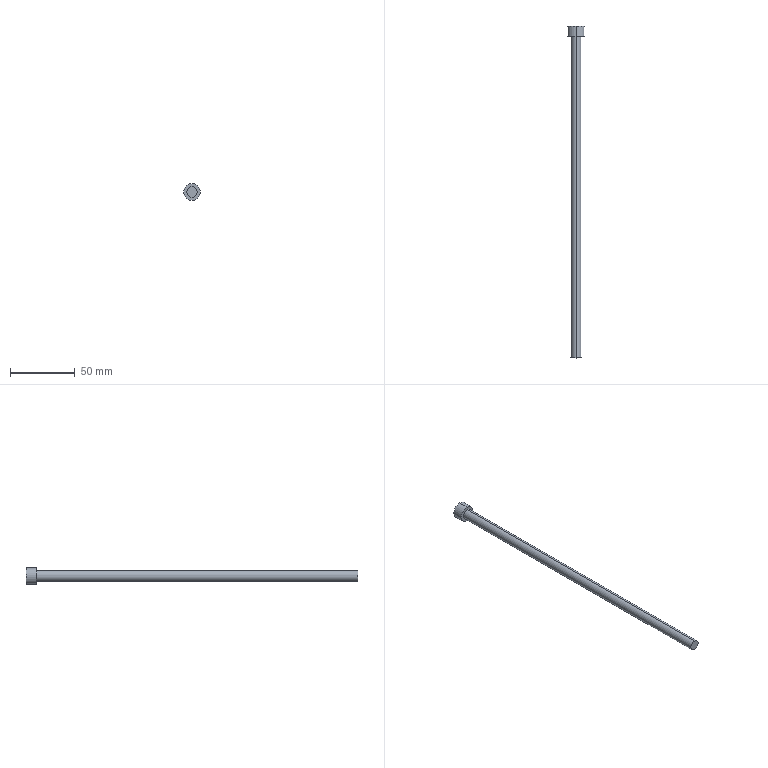Part | STEP file | 1 solid | 7 faces | box 13 x 257.335 x 13 mm | volume 13595 mm3 | cylinder 4 | plane 3 | commonest cylinder face diameters 8 x2 13 x2
STEP:
#1=CARTESIAN_POINT('',(0.,0.,0.));
#2=DIRECTION('',(0.,0.,1.));
#3=DIRECTION('',(1.,0.,0.));
#4=AXIS2_PLACEMENT_3D('',#1,#2,#3);
#5=CARTESIAN_POINT('',(-72.861,290.5,9.027));
#6=VERTEX_POINT('',#5);
#7=CARTESIAN_POINT('',(-72.861,290.5,22.027));
#8=VERTEX_POINT('',#7);
#9=CARTESIAN_POINT('',(-72.861,290.5,15.527));
#10=DIRECTION('',(0.,-1.,0.));
#11=DIRECTION('',(0.,0.,-1.));
#12=AXIS2_PLACEMENT_3D('',#9,#10,#11);
#13=CIRCLE('',#12,6.5);
#14=CARTESIAN_POINT('',(-72.861,290.5,15.527));
#15=DIRECTION('',(0.,-1.,0.));
#16=DIRECTION('',(0.,0.,-1.));
#17=AXIS2_PLACEMENT_3D('',#14,#15,#16);
#18=CYLINDRICAL_SURFACE('',#17,6.5);
#19=CARTESIAN_POINT('',(0.,0.));
#20=DIRECTION('',(1.,0.));
#21=VECTOR('',#20,1.);
#22=LINE('',#19,#21);
#23=(GEOMETRIC_REPRESENTATION_CONTEXT(2)PARAMETRIC_REPRESENTATION_CONTEXT()REPRESENTATION_CONTEXT('',''));
#24=DEFINITIONAL_REPRESENTATION('',(#22),#23);
#25=PCURVE('',#18,#24);
#26=CARTESIAN_POINT('',(-72.862,290.5,110.196));
#27=DIRECTION('',(0.,-1.,0.));
#28=DIRECTION('',(0.,0.,-1.));
#29=AXIS2_PLACEMENT_3D('',#26,#27,#28);
#30=PLANE('',#29);
#31=CARTESIAN_POINT('',(94.669,0.00185));
#32=DIRECTION('',(1.,0.));
#33=AXIS2_PLACEMENT_2D('',#31,#32);
#34=CIRCLE('',#33,6.5);
#35=(GEOMETRIC_REPRESENTATION_CONTEXT(2)PARAMETRIC_REPRESENTATION_CONTEXT()REPRESENTATION_CONTEXT('',''));
#36=DEFINITIONAL_REPRESENTATION('',(#34),#35);
#37=PCURVE('',#30,#36);
#38=SURFACE_CURVE('',#13,(#25,#37),.PCURVE_S1.);
#39=EDGE_CURVE('',#6,#8,#38,.T.);
#40=ORIENTED_EDGE('',*,*,#39,.T.);
#41=CARTESIAN_POINT('',(-72.861,282.5,22.027));
#42=VERTEX_POINT('',#41);
#43=CARTESIAN_POINT('',(-72.861,290.5,22.027));
#44=DIRECTION('',(0.,-1.,0.));
#45=VECTOR('',#44,1.);
#46=LINE('',#43,#45);
#47=CARTESIAN_POINT('',(3.142,0.));
#48=DIRECTION('',(0.,1.));
#49=VECTOR('',#48,1.);
#50=LINE('',#47,#49);
#51=(GEOMETRIC_REPRESENTATION_CONTEXT(2)PARAMETRIC_REPRESENTATION_CONTEXT()REPRESENTATION_CONTEXT('',''));
#52=DEFINITIONAL_REPRESENTATION('',(#50),#51);
#53=PCURVE('',#18,#52);
#54=CARTESIAN_POINT('',(-72.861,290.5,15.527));
#55=DIRECTION('',(0.,-1.,0.));
#56=DIRECTION('',(0.,0.,-1.));
#57=AXIS2_PLACEMENT_3D('',#54,#55,#56);
#58=CYLINDRICAL_SURFACE('',#57,6.5);
#59=CARTESIAN_POINT('',(3.142,0.));
#60=DIRECTION('',(0.,1.));
#61=VECTOR('',#60,1.);
#62=LINE('',#59,#61);
#63=(GEOMETRIC_REPRESENTATION_CONTEXT(2)PARAMETRIC_REPRESENTATION_CONTEXT()REPRESENTATION_CONTEXT('',''));
#64=DEFINITIONAL_REPRESENTATION('',(#62),#63);
#65=PCURVE('',#58,#64);
#66=SURFACE_CURVE('',#46,(#53,#65),.PCURVE_S1.);
#67=EDGE_CURVE('',#8,#42,#66,.T.);
#68=ORIENTED_EDGE('',*,*,#67,.T.);
#69=CARTESIAN_POINT('',(-72.861,282.5,9.027));
#70=VERTEX_POINT('',#69);
#71=CARTESIAN_POINT('',(-72.861,282.5,15.527));
#72=DIRECTION('',(0.,1.,0.));
#73=DIRECTION('',(0.,0.,1.));
#74=AXIS2_PLACEMENT_3D('',#71,#72,#73);
#75=CIRCLE('',#74,6.5);
#76=CARTESIAN_POINT('',(3.142,8.));
#77=DIRECTION('',(-1.,0.));
#78=VECTOR('',#77,1.);
#79=LINE('',#76,#78);
#80=(GEOMETRIC_REPRESENTATION_CONTEXT(2)PARAMETRIC_REPRESENTATION_CONTEXT()REPRESENTATION_CONTEXT('',''));
#81=DEFINITIONAL_REPRESENTATION('',(#79),#80);
#82=PCURVE('',#18,#81);
#83=CARTESIAN_POINT('',(-72.861,282.5,15.527));
#84=DIRECTION('',(0.,-1.,0.));
#85=DIRECTION('',(0.,0.,-1.));
#86=AXIS2_PLACEMENT_3D('',#83,#84,#85);
#87=PLANE('',#86);
#88=CARTESIAN_POINT('',(-6.5,0.));
#89=CARTESIAN_POINT('',(-6.5,11.258));
#90=CARTESIAN_POINT('',(3.25,5.629));
#91=CARTESIAN_POINT('',(13.,0.));
#92=CARTESIAN_POINT('',(3.25,-5.629));
#93=CARTESIAN_POINT('',(-6.5,-11.258));
#94=CARTESIAN_POINT('',(-6.5,0.));
#95=(BOUNDED_CURVE()B_SPLINE_CURVE(2,(#88,#89,#90,#91,#92,#93,#94),.UNSPECIFIED.,.T.,.F.)B_SPLINE_CURVE_WITH_KNOTS((1,2,2,2,2,1),(-2.094,0.,2.094,4.189,6.283,8.378),.UNSPECIFIED.)CURVE()GEOMETRIC_REPRESENTATION_ITEM()RATIONAL_B_SPLINE_CURVE((1.,0.5,1.,0.5,1.,0.5,1.))REPRESENTATION_ITEM(''));
#96=(GEOMETRIC_REPRESENTATION_CONTEXT(2)PARAMETRIC_REPRESENTATION_CONTEXT()REPRESENTATION_CONTEXT('',''));
#97=DEFINITIONAL_REPRESENTATION('',(#95),#96);
#98=PCURVE('',#87,#97);
#99=SURFACE_CURVE('',#75,(#82,#98),.PCURVE_S1.);
#100=EDGE_CURVE('',#42,#70,#99,.T.);
#101=ORIENTED_EDGE('',*,*,#100,.T.);
#102=CARTESIAN_POINT('',(-72.861,290.5,9.027));
#103=DIRECTION('',(0.,-1.,0.));
#104=VECTOR('',#103,1.);
#105=LINE('',#102,#104);
#106=CARTESIAN_POINT('',(0.,0.));
#107=DIRECTION('',(0.,1.));
#108=VECTOR('',#107,1.);
#109=LINE('',#106,#108);
#110=(GEOMETRIC_REPRESENTATION_CONTEXT(2)PARAMETRIC_REPRESENTATION_CONTEXT()REPRESENTATION_CONTEXT('',''));
#111=DEFINITIONAL_REPRESENTATION('',(#109),#110);
#112=PCURVE('',#18,#111);
#113=CARTESIAN_POINT('',(6.283,0.));
#114=DIRECTION('',(0.,1.));
#115=VECTOR('',#114,1.);
#116=LINE('',#113,#115);
#117=(GEOMETRIC_REPRESENTATION_CONTEXT(2)PARAMETRIC_REPRESENTATION_CONTEXT()REPRESENTATION_CONTEXT('',''));
#118=DEFINITIONAL_REPRESENTATION('',(#116),#117);
#119=PCURVE('',#58,#118);
#120=SURFACE_CURVE('',#105,(#112,#119),.PCURVE_S1.);
#121=EDGE_CURVE('',#6,#70,#120,.T.);
#122=ORIENTED_EDGE('',*,*,#121,.F.);
#123=EDGE_LOOP('',(#40,#68,#101,#122));
#124=FACE_BOUND('',#123,.T.);
#125=ADVANCED_FACE('',(#124),#18,.T.);
#126=CARTESIAN_POINT('',(-72.861,282.5,19.527));
#127=VERTEX_POINT('',#126);
#128=CARTESIAN_POINT('',(-72.861,282.5,11.527));
#129=VERTEX_POINT('',#128);
#130=CARTESIAN_POINT('',(-72.861,282.5,15.527));
#131=DIRECTION('',(0.,1.,0.));
#132=DIRECTION('',(0.,0.,-1.));
#133=AXIS2_PLACEMENT_3D('',#130,#131,#132);
#134=CIRCLE('',#133,4.);
#135=CARTESIAN_POINT('',(-72.861,220.5,15.527));
#136=DIRECTION('',(0.,-1.,0.));
#137=DIRECTION('',(0.,0.,-1.));
#138=AXIS2_PLACEMENT_3D('',#135,#136,#137);
#139=CYLINDRICAL_SURFACE('',#138,4.);
#140=CARTESIAN_POINT('',(6.283,-62.));
#141=DIRECTION('',(-1.,0.));
#142=VECTOR('',#141,1.);
#143=LINE('',#140,#142);
#144=(GEOMETRIC_REPRESENTATION_CONTEXT(2)PARAMETRIC_REPRESENTATION_CONTEXT()REPRESENTATION_CONTEXT('',''));
#145=DEFINITIONAL_REPRESENTATION('',(#143),#144);
#146=PCURVE('',#139,#145);
#147=CARTESIAN_POINT('',(4.,0.));
#148=CARTESIAN_POINT('',(4.,-6.928));
#149=CARTESIAN_POINT('',(-2.,-3.464));
#150=CARTESIAN_POINT('',(-8.,0.));
#151=CARTESIAN_POINT('',(-2.,3.464));
#152=CARTESIAN_POINT('',(4.,6.928));
#153=CARTESIAN_POINT('',(4.,0.));
#154=(BOUNDED_CURVE()B_SPLINE_CURVE(2,(#147,#148,#149,#150,#151,#152,#153),.UNSPECIFIED.,.T.,.F.)B_SPLINE_CURVE_WITH_KNOTS((1,2,2,2,2,1),(-2.094,0.,2.094,4.189,6.283,8.378),.UNSPECIFIED.)CURVE()GEOMETRIC_REPRESENTATION_ITEM()RATIONAL_B_SPLINE_CURVE((1.,0.5,1.,0.5,1.,0.5,1.))REPRESENTATION_ITEM(''));
#155=(GEOMETRIC_REPRESENTATION_CONTEXT(2)PARAMETRIC_REPRESENTATION_CONTEXT()REPRESENTATION_CONTEXT('',''));
#156=DEFINITIONAL_REPRESENTATION('',(#154),#155);
#157=PCURVE('',#87,#156);
#158=SURFACE_CURVE('',#134,(#146,#157),.PCURVE_S1.);
#159=EDGE_CURVE('',#127,#129,#158,.T.);
#160=ORIENTED_EDGE('',*,*,#159,.F.);
#161=CARTESIAN_POINT('',(-72.861,33.165,19.527));
#162=VERTEX_POINT('',#161);
#163=CARTESIAN_POINT('',(-72.861,220.5,19.527));
#164=DIRECTION('',(0.,-1.,0.));
#165=VECTOR('',#164,1.);
#166=LINE('',#163,#165);
#167=CARTESIAN_POINT('',(3.142,0.));
#168=DIRECTION('',(0.,1.));
#169=VECTOR('',#168,1.);
#170=LINE('',#167,#169);
#171=(GEOMETRIC_REPRESENTATION_CONTEXT(2)PARAMETRIC_REPRESENTATION_CONTEXT()REPRESENTATION_CONTEXT('',''));
#172=DEFINITIONAL_REPRESENTATION('',(#170),#171);
#173=PCURVE('',#139,#172);
#174=CARTESIAN_POINT('',(-72.861,220.5,15.527));
#175=DIRECTION('',(0.,-1.,0.));
#176=DIRECTION('',(0.,0.,-1.));
#177=AXIS2_PLACEMENT_3D('',#174,#175,#176);
#178=CYLINDRICAL_SURFACE('',#177,4.);
#179=CARTESIAN_POINT('',(3.142,0.));
#180=DIRECTION('',(0.,1.));
#181=VECTOR('',#180,1.);
#182=LINE('',#179,#181);
#183=(GEOMETRIC_REPRESENTATION_CONTEXT(2)PARAMETRIC_REPRESENTATION_CONTEXT()REPRESENTATION_CONTEXT('',''));
#184=DEFINITIONAL_REPRESENTATION('',(#182),#183);
#185=PCURVE('',#178,#184);
#186=SURFACE_CURVE('',#166,(#173,#185),.PCURVE_S1.);
#187=EDGE_CURVE('',#127,#162,#186,.T.);
#188=ORIENTED_EDGE('',*,*,#187,.T.);
#189=CARTESIAN_POINT('',(-72.861,33.165,11.527));
#190=VERTEX_POINT('',#189);
#191=CARTESIAN_POINT('',(-72.861,33.165,15.527));
#192=DIRECTION('',(0.,1.,0.));
#193=DIRECTION('',(0.,0.,-1.));
#194=AXIS2_PLACEMENT_3D('',#191,#192,#193);
#195=CIRCLE('',#194,4.);
#196=CARTESIAN_POINT('',(6.283,187.335));
#197=DIRECTION('',(-1.,0.));
#198=VECTOR('',#197,1.);
#199=LINE('',#196,#198);
#200=(GEOMETRIC_REPRESENTATION_CONTEXT(2)PARAMETRIC_REPRESENTATION_CONTEXT()REPRESENTATION_CONTEXT('',''));
#201=DEFINITIONAL_REPRESENTATION('',(#199),#200);
#202=PCURVE('',#139,#201);
#203=CARTESIAN_POINT('',(-4.271,33.165,10.143));
#204=DIRECTION('',(0.,-1.,0.));
#205=DIRECTION('',(0.,0.,-1.));
#206=AXIS2_PLACEMENT_3D('',#203,#204,#205);
#207=PLANE('',#206);
#208=CARTESIAN_POINT('',(-1.384,-68.589));
#209=CARTESIAN_POINT('',(-1.384,-75.518));
#210=CARTESIAN_POINT('',(-7.384,-72.054));
#211=CARTESIAN_POINT('',(-13.384,-68.589));
#212=CARTESIAN_POINT('',(-7.384,-65.125));
#213=CARTESIAN_POINT('',(-1.384,-61.661));
#214=CARTESIAN_POINT('',(-1.384,-68.589));
#215=(BOUNDED_CURVE()B_SPLINE_CURVE(2,(#208,#209,#210,#211,#212,#213,#214),.UNSPECIFIED.,.T.,.F.)B_SPLINE_CURVE_WITH_KNOTS((1,2,2,2,2,1),(-2.094,0.,2.094,4.189,6.283,8.378),.UNSPECIFIED.)CURVE()GEOMETRIC_REPRESENTATION_ITEM()RATIONAL_B_SPLINE_CURVE((1.,0.5,1.,0.5,1.,0.5,1.))REPRESENTATION_ITEM(''));
#216=(GEOMETRIC_REPRESENTATION_CONTEXT(2)PARAMETRIC_REPRESENTATION_CONTEXT()REPRESENTATION_CONTEXT('',''));
#217=DEFINITIONAL_REPRESENTATION('',(#215),#216);
#218=PCURVE('',#207,#217);
#219=SURFACE_CURVE('',#195,(#202,#218),.PCURVE_S1.);
#220=EDGE_CURVE('',#162,#190,#219,.T.);
#221=ORIENTED_EDGE('',*,*,#220,.T.);
#222=CARTESIAN_POINT('',(-72.861,220.5,11.527));
#223=DIRECTION('',(0.,-1.,0.));
#224=VECTOR('',#223,1.);
#225=LINE('',#222,#224);
#226=CARTESIAN_POINT('',(0.,0.));
#227=DIRECTION('',(0.,1.));
#228=VECTOR('',#227,1.);
#229=LINE('',#226,#228);
#230=(GEOMETRIC_REPRESENTATION_CONTEXT(2)PARAMETRIC_REPRESENTATION_CONTEXT()REPRESENTATION_CONTEXT('',''));
#231=DEFINITIONAL_REPRESENTATION('',(#229),#230);
#232=PCURVE('',#139,#231);
#233=CARTESIAN_POINT('',(6.283,0.));
#234=DIRECTION('',(0.,1.));
#235=VECTOR('',#234,1.);
#236=LINE('',#233,#235);
#237=(GEOMETRIC_REPRESENTATION_CONTEXT(2)PARAMETRIC_REPRESENTATION_CONTEXT()REPRESENTATION_CONTEXT('',''));
#238=DEFINITIONAL_REPRESENTATION('',(#236),#237);
#239=PCURVE('',#178,#238);
#240=SURFACE_CURVE('',#225,(#232,#239),.PCURVE_S1.);
#241=EDGE_CURVE('',#129,#190,#240,.T.);
#242=ORIENTED_EDGE('',*,*,#241,.F.);
#243=EDGE_LOOP('',(#160,#188,#221,#242));
#244=FACE_BOUND('',#243,.T.);
#245=ADVANCED_FACE('',(#244),#139,.T.);
#246=ORIENTED_EDGE('',*,*,#187,.F.);
#247=CARTESIAN_POINT('',(-72.861,282.5,15.527));
#248=DIRECTION('',(0.,1.,0.));
#249=DIRECTION('',(0.,0.,-1.));
#250=AXIS2_PLACEMENT_3D('',#247,#248,#249);
#251=CIRCLE('',#250,4.);
#252=CARTESIAN_POINT('',(6.283,-62.));
#253=DIRECTION('',(-1.,0.));
#254=VECTOR('',#253,1.);
#255=LINE('',#252,#254);
#256=(GEOMETRIC_REPRESENTATION_CONTEXT(2)PARAMETRIC_REPRESENTATION_CONTEXT()REPRESENTATION_CONTEXT('',''));
#257=DEFINITIONAL_REPRESENTATION('',(#255),#256);
#258=PCURVE('',#178,#257);
#259=CARTESIAN_POINT('',(4.,0.));
#260=CARTESIAN_POINT('',(4.,-6.928));
#261=CARTESIAN_POINT('',(-2.,-3.464));
#262=CARTESIAN_POINT('',(-8.,0.));
#263=CARTESIAN_POINT('',(-2.,3.464));
#264=CARTESIAN_POINT('',(4.,6.928));
#265=CARTESIAN_POINT('',(4.,0.));
#266=(BOUNDED_CURVE()B_SPLINE_CURVE(2,(#259,#260,#261,#262,#263,#264,#265),.UNSPECIFIED.,.T.,.F.)B_SPLINE_CURVE_WITH_KNOTS((1,2,2,2,2,1),(-2.094,0.,2.094,4.189,6.283,8.378),.UNSPECIFIED.)CURVE()GEOMETRIC_REPRESENTATION_ITEM()RATIONAL_B_SPLINE_CURVE((1.,0.5,1.,0.5,1.,0.5,1.))REPRESENTATION_ITEM(''));
#267=(GEOMETRIC_REPRESENTATION_CONTEXT(2)PARAMETRIC_REPRESENTATION_CONTEXT()REPRESENTATION_CONTEXT('',''));
#268=DEFINITIONAL_REPRESENTATION('',(#266),#267);
#269=PCURVE('',#87,#268);
#270=SURFACE_CURVE('',#251,(#258,#269),.PCURVE_S1.);
#271=EDGE_CURVE('',#129,#127,#270,.T.);
#272=ORIENTED_EDGE('',*,*,#271,.F.);
#273=ORIENTED_EDGE('',*,*,#241,.T.);
#274=CARTESIAN_POINT('',(-72.861,33.165,15.527));
#275=DIRECTION('',(0.,1.,0.));
#276=DIRECTION('',(0.,0.,-1.));
#277=AXIS2_PLACEMENT_3D('',#274,#275,#276);
#278=CIRCLE('',#277,4.);
#279=CARTESIAN_POINT('',(6.283,187.335));
#280=DIRECTION('',(-1.,0.));
#281=VECTOR('',#280,1.);
#282=LINE('',#279,#281);
#283=(GEOMETRIC_REPRESENTATION_CONTEXT(2)PARAMETRIC_REPRESENTATION_CONTEXT()REPRESENTATION_CONTEXT('',''));
#284=DEFINITIONAL_REPRESENTATION('',(#282),#283);
#285=PCURVE('',#178,#284);
#286=CARTESIAN_POINT('',(-1.384,-68.589));
#287=CARTESIAN_POINT('',(-1.384,-75.518));
#288=CARTESIAN_POINT('',(-7.384,-72.054));
#289=CARTESIAN_POINT('',(-13.384,-68.589));
#290=CARTESIAN_POINT('',(-7.384,-65.125));
#291=CARTESIAN_POINT('',(-1.384,-61.661));
#292=CARTESIAN_POINT('',(-1.384,-68.589));
#293=(BOUNDED_CURVE()B_SPLINE_CURVE(2,(#286,#287,#288,#289,#290,#291,#292),.UNSPECIFIED.,.T.,.F.)B_SPLINE_CURVE_WITH_KNOTS((1,2,2,2,2,1),(-2.094,0.,2.094,4.189,6.283,8.378),.UNSPECIFIED.)CURVE()GEOMETRIC_REPRESENTATION_ITEM()RATIONAL_B_SPLINE_CURVE((1.,0.5,1.,0.5,1.,0.5,1.))REPRESENTATION_ITEM(''));
#294=(GEOMETRIC_REPRESENTATION_CONTEXT(2)PARAMETRIC_REPRESENTATION_CONTEXT()REPRESENTATION_CONTEXT('',''));
#295=DEFINITIONAL_REPRESENTATION('',(#293),#294);
#296=PCURVE('',#207,#295);
#297=SURFACE_CURVE('',#278,(#285,#296),.PCURVE_S1.);
#298=EDGE_CURVE('',#190,#162,#297,.T.);
#299=ORIENTED_EDGE('',*,*,#298,.T.);
#300=EDGE_LOOP('',(#246,#272,#273,#299));
#301=FACE_BOUND('',#300,.T.);
#302=ADVANCED_FACE('',(#301),#178,.T.);
#303=ORIENTED_EDGE('',*,*,#298,.F.);
#304=ORIENTED_EDGE('',*,*,#220,.F.);
#305=EDGE_LOOP('',(#303,#304));
#306=FACE_BOUND('',#305,.T.);
#307=ADVANCED_FACE('',(#306),#207,.T.);
#308=ORIENTED_EDGE('',*,*,#271,.T.);
#309=ORIENTED_EDGE('',*,*,#159,.T.);
#310=EDGE_LOOP('',(#308,#309));
#311=FACE_BOUND('',#310,.T.);
#312=CARTESIAN_POINT('',(-72.861,282.5,15.527));
#313=DIRECTION('',(0.,1.,0.));
#314=DIRECTION('',(0.,0.,1.));
#315=AXIS2_PLACEMENT_3D('',#312,#313,#314);
#316=CIRCLE('',#315,6.5);
#317=CARTESIAN_POINT('',(-6.5,0.));
#318=CARTESIAN_POINT('',(-6.5,11.258));
#319=CARTESIAN_POINT('',(3.25,5.629));
#320=CARTESIAN_POINT('',(13.,0.));
#321=CARTESIAN_POINT('',(3.25,-5.629));
#322=CARTESIAN_POINT('',(-6.5,-11.258));
#323=CARTESIAN_POINT('',(-6.5,0.));
#324=(BOUNDED_CURVE()B_SPLINE_CURVE(2,(#317,#318,#319,#320,#321,#322,#323),.UNSPECIFIED.,.T.,.F.)B_SPLINE_CURVE_WITH_KNOTS((1,2,2,2,2,1),(-2.094,0.,2.094,4.189,6.283,8.378),.UNSPECIFIED.)CURVE()GEOMETRIC_REPRESENTATION_ITEM()RATIONAL_B_SPLINE_CURVE((1.,0.5,1.,0.5,1.,0.5,1.))REPRESENTATION_ITEM(''));
#325=(GEOMETRIC_REPRESENTATION_CONTEXT(2)PARAMETRIC_REPRESENTATION_CONTEXT()REPRESENTATION_CONTEXT('',''));
#326=DEFINITIONAL_REPRESENTATION('',(#324),#325);
#327=PCURVE('',#87,#326);
#328=CARTESIAN_POINT('',(9.425,8.));
#329=DIRECTION('',(-1.,0.));
#330=VECTOR('',#329,1.);
#331=LINE('',#328,#330);
#332=(GEOMETRIC_REPRESENTATION_CONTEXT(2)PARAMETRIC_REPRESENTATION_CONTEXT()REPRESENTATION_CONTEXT('',''));
#333=DEFINITIONAL_REPRESENTATION('',(#331),#332);
#334=PCURVE('',#58,#333);
#335=SURFACE_CURVE('',#316,(#327,#334),.PCURVE_S1.);
#336=EDGE_CURVE('',#70,#42,#335,.T.);
#337=ORIENTED_EDGE('',*,*,#336,.F.);
#338=ORIENTED_EDGE('',*,*,#100,.F.);
#339=EDGE_LOOP('',(#337,#338));
#340=FACE_BOUND('',#339,.T.);
#341=ADVANCED_FACE('',(#311,#340),#87,.T.);
#342=ORIENTED_EDGE('',*,*,#67,.F.);
#343=CARTESIAN_POINT('',(-72.861,290.5,15.527));
#344=DIRECTION('',(0.,-1.,0.));
#345=DIRECTION('',(0.,0.,-1.));
#346=AXIS2_PLACEMENT_3D('',#343,#344,#345);
#347=CIRCLE('',#346,6.5);
#348=CARTESIAN_POINT('',(0.,0.));
#349=DIRECTION('',(1.,0.));
#350=VECTOR('',#349,1.);
#351=LINE('',#348,#350);
#352=(GEOMETRIC_REPRESENTATION_CONTEXT(2)PARAMETRIC_REPRESENTATION_CONTEXT()REPRESENTATION_CONTEXT('',''));
#353=DEFINITIONAL_REPRESENTATION('',(#351),#352);
#354=PCURVE('',#58,#353);
#355=CARTESIAN_POINT('',(94.669,0.00185));
#356=DIRECTION('',(1.,0.));
#357=AXIS2_PLACEMENT_2D('',#355,#356);
#358=CIRCLE('',#357,6.5);
#359=(GEOMETRIC_REPRESENTATION_CONTEXT(2)PARAMETRIC_REPRESENTATION_CONTEXT()REPRESENTATION_CONTEXT('',''));
#360=DEFINITIONAL_REPRESENTATION('',(#358),#359);
#361=PCURVE('',#30,#360);
#362=SURFACE_CURVE('',#347,(#354,#361),.PCURVE_S1.);
#363=EDGE_CURVE('',#8,#6,#362,.T.);
#364=ORIENTED_EDGE('',*,*,#363,.T.);
#365=ORIENTED_EDGE('',*,*,#121,.T.);
#366=ORIENTED_EDGE('',*,*,#336,.T.);
#367=EDGE_LOOP('',(#342,#364,#365,#366));
#368=FACE_BOUND('',#367,.T.);
#369=ADVANCED_FACE('',(#368),#58,.T.);
#370=ORIENTED_EDGE('',*,*,#39,.F.);
#371=ORIENTED_EDGE('',*,*,#363,.F.);
#372=EDGE_LOOP('',(#370,#371));
#373=FACE_BOUND('',#372,.T.);
#374=ADVANCED_FACE('',(#373),#30,.F.);
#375=CLOSED_SHELL('',(#125,#245,#302,#307,#341,#369,#374));
#376=MANIFOLD_SOLID_BREP('',#375);
#377=(LENGTH_UNIT()NAMED_UNIT(*)SI_UNIT(.MILLI.,.METRE.));
#378=UNCERTAINTY_MEASURE_WITH_UNIT(LENGTH_MEASURE(0.0000001),#377,'','');
#379=(NAMED_UNIT(*)PLANE_ANGLE_UNIT()SI_UNIT($,.RADIAN.));
#380=(NAMED_UNIT(*)SI_UNIT($,.STERADIAN.)SOLID_ANGLE_UNIT());
#381=(GEOMETRIC_REPRESENTATION_CONTEXT(3)GLOBAL_UNCERTAINTY_ASSIGNED_CONTEXT((#378))GLOBAL_UNIT_ASSIGNED_CONTEXT((#377,#379,#380))REPRESENTATION_CONTEXT('',''));
#382=ADVANCED_BREP_SHAPE_REPRESENTATION('',(#4,#376),#381);